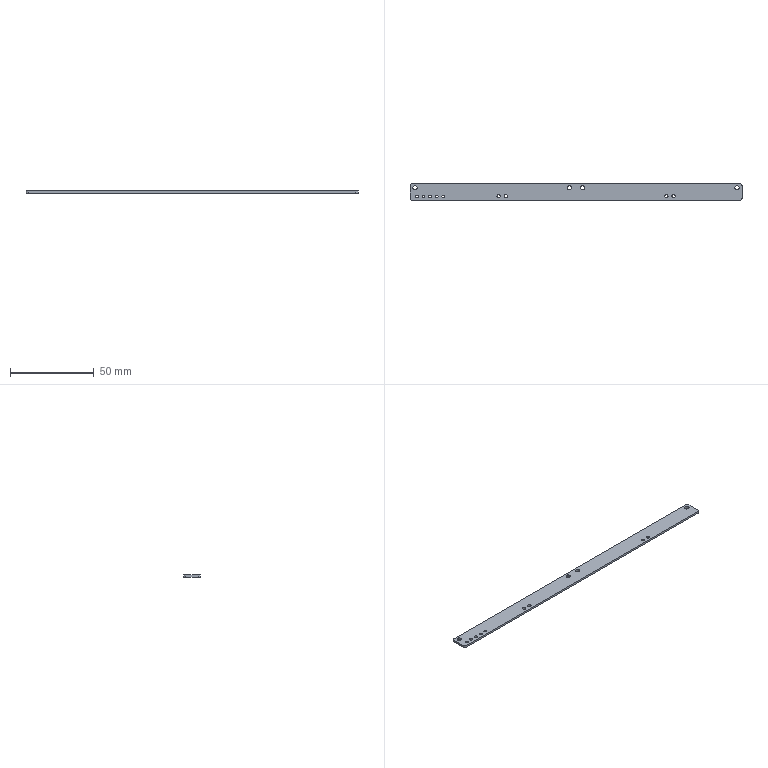Part | STEP file | Power supply board | 1 solid | 23 faces | box 198 x 10 x 1.2 mm | volume 2320 mm3 | cylinder 17 | plane 6 | commonest cylinder face diameters 1.7 x5 2 x4 2.54 x4 2.6 x4